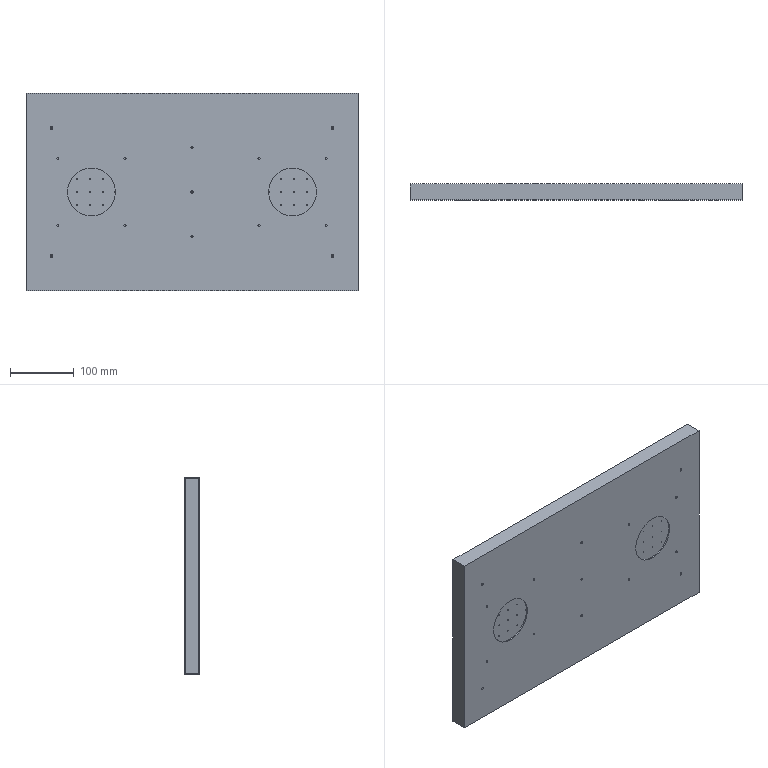Part | SolidWorks | features BaseBody 1 | 1 solid | 841 faces | box 520 x 25 x 310 mm | volume 696143 mm3 | cylinder 814 | plane 27 | commonest cylinder face diameters 1.5 x750 3.3 x22 7.9 x22 4.2 x8 8.7 x8 75 x4